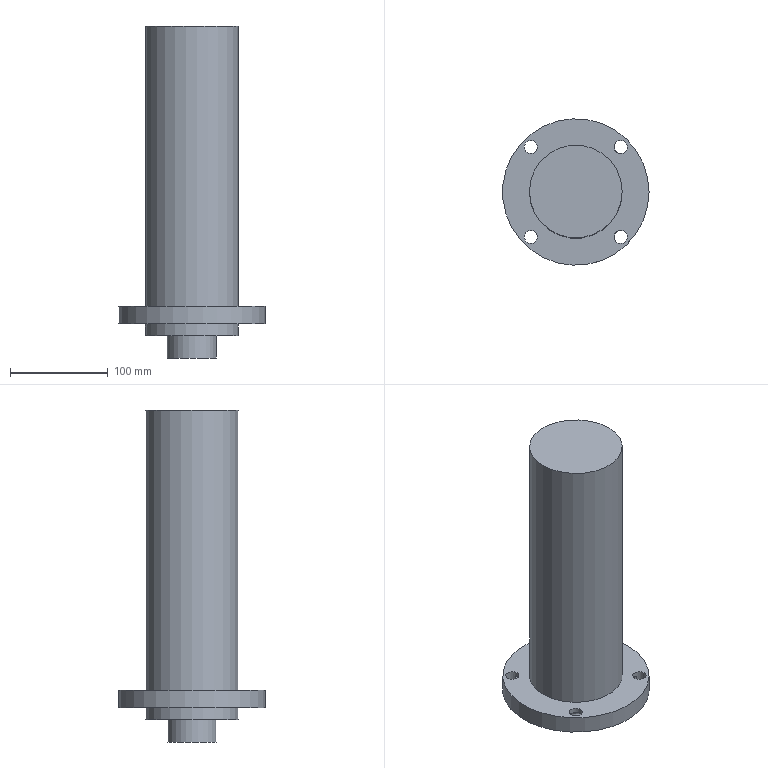Part | NX | features solid 2 | 1 solid | 14 faces | box 150 x 150 x 340 mm | volume 2465510 mm3 | cylinder 8 | plane 5 | torus 1 | commonest cylinder face diameters 13.5 x4 95 x2 50 x1 150 x1
STEP:
#1=CARTESIAN_POINT('',(955.75,441.,55.));
#2=VERTEX_POINT('',#1);
#3=CARTESIAN_POINT('',(949.,441.,55.));
#4=DIRECTION('',(0.,0.,1.));
#5=DIRECTION('',(1.,0.,0.));
#6=AXIS2_PLACEMENT_3D('',#3,#4,#5);
#7=CIRCLE('',#6,6.75);
#8=EDGE_CURVE('',#2,#2,#7,.F.);
#9=ORIENTED_EDGE('',*,*,#8,.T.);
#10=EDGE_LOOP('',(#9));
#11=FACE_BOUND('',#10,.T.);
#12=CARTESIAN_POINT('',(1047.75,349.,55.));
#13=VERTEX_POINT('',#12);
#14=CARTESIAN_POINT('',(1041.,349.,55.));
#15=DIRECTION('',(0.,0.,1.));
#16=DIRECTION('',(1.,0.,0.));
#17=AXIS2_PLACEMENT_3D('',#14,#15,#16);
#18=CIRCLE('',#17,6.75);
#19=EDGE_CURVE('',#13,#13,#18,.F.);
#20=ORIENTED_EDGE('',*,*,#19,.T.);
#21=EDGE_LOOP('',(#20));
#22=FACE_BOUND('',#21,.T.);
#23=CARTESIAN_POINT('',(1070.,395.,55.));
#24=VERTEX_POINT('',#23);
#25=CARTESIAN_POINT('',(995.,395.,55.));
#26=DIRECTION('',(0.,0.,1.));
#27=DIRECTION('',(1.,0.,0.));
#28=AXIS2_PLACEMENT_3D('',#25,#26,#27);
#29=CIRCLE('',#28,75.);
#30=EDGE_CURVE('',#24,#24,#29,.T.);
#31=ORIENTED_EDGE('',*,*,#30,.T.);
#32=EDGE_LOOP('',(#31));
#33=FACE_BOUND('',#32,.T.);
#34=CARTESIAN_POINT('',(1042.5,395.,55.));
#35=VERTEX_POINT('',#34);
#36=CARTESIAN_POINT('',(995.,395.,55.));
#37=DIRECTION('',(0.,0.,1.));
#38=DIRECTION('',(1.,0.,0.));
#39=AXIS2_PLACEMENT_3D('',#36,#37,#38);
#40=CIRCLE('',#39,47.5);
#41=EDGE_CURVE('',#35,#35,#40,.T.);
#42=ORIENTED_EDGE('',*,*,#41,.F.);
#43=EDGE_LOOP('',(#42));
#44=FACE_BOUND('',#43,.T.);
#45=CARTESIAN_POINT('',(1047.75,441.,55.));
#46=VERTEX_POINT('',#45);
#47=CARTESIAN_POINT('',(1041.,441.,55.));
#48=DIRECTION('',(0.,0.,1.));
#49=DIRECTION('',(1.,0.,0.));
#50=AXIS2_PLACEMENT_3D('',#47,#48,#49);
#51=CIRCLE('',#50,6.75);
#52=EDGE_CURVE('',#46,#46,#51,.F.);
#53=ORIENTED_EDGE('',*,*,#52,.T.);
#54=EDGE_LOOP('',(#53));
#55=FACE_BOUND('',#54,.T.);
#56=CARTESIAN_POINT('',(955.75,349.,55.));
#57=VERTEX_POINT('',#56);
#58=CARTESIAN_POINT('',(949.,349.,55.));
#59=DIRECTION('',(0.,0.,1.));
#60=DIRECTION('',(1.,0.,0.));
#61=AXIS2_PLACEMENT_3D('',#58,#59,#60);
#62=CIRCLE('',#61,6.75);
#63=EDGE_CURVE('',#57,#57,#62,.F.);
#64=ORIENTED_EDGE('',*,*,#63,.T.);
#65=EDGE_LOOP('',(#64));
#66=FACE_BOUND('',#65,.T.);
#67=CARTESIAN_POINT('',(995.,395.,55.));
#68=DIRECTION('',(0.,0.,-1.));
#69=DIRECTION('',(1.,0.,0.));
#70=AXIS2_PLACEMENT_3D('',#67,#68,#69);
#71=PLANE('',#70);
#72=ADVANCED_FACE('',(#11,#22,#33,#44,#55,#66),#71,.F.);
#73=CARTESIAN_POINT('',(955.75,441.,37.));
#74=VERTEX_POINT('',#73);
#75=CARTESIAN_POINT('',(949.,441.,37.));
#76=DIRECTION('',(0.,0.,1.));
#77=DIRECTION('',(1.,0.,0.));
#78=AXIS2_PLACEMENT_3D('',#75,#76,#77);
#79=CIRCLE('',#78,6.75);
#80=EDGE_CURVE('',#74,#74,#79,.F.);
#81=ORIENTED_EDGE('',*,*,#80,.F.);
#82=EDGE_LOOP('',(#81));
#83=FACE_BOUND('',#82,.T.);
#84=CARTESIAN_POINT('',(1047.75,349.,37.));
#85=VERTEX_POINT('',#84);
#86=CARTESIAN_POINT('',(1041.,349.,37.));
#87=DIRECTION('',(0.,0.,1.));
#88=DIRECTION('',(1.,0.,0.));
#89=AXIS2_PLACEMENT_3D('',#86,#87,#88);
#90=CIRCLE('',#89,6.75);
#91=EDGE_CURVE('',#85,#85,#90,.F.);
#92=ORIENTED_EDGE('',*,*,#91,.F.);
#93=EDGE_LOOP('',(#92));
#94=FACE_BOUND('',#93,.T.);
#95=CARTESIAN_POINT('',(1070.,395.,37.));
#96=VERTEX_POINT('',#95);
#97=CARTESIAN_POINT('',(995.,395.,37.));
#98=DIRECTION('',(0.,0.,1.));
#99=DIRECTION('',(1.,0.,0.));
#100=AXIS2_PLACEMENT_3D('',#97,#98,#99);
#101=CIRCLE('',#100,75.);
#102=EDGE_CURVE('',#96,#96,#101,.T.);
#103=ORIENTED_EDGE('',*,*,#102,.F.);
#104=EDGE_LOOP('',(#103));
#105=FACE_BOUND('',#104,.T.);
#106=CARTESIAN_POINT('',(1042.5,395.,37.));
#107=VERTEX_POINT('',#106);
#108=CARTESIAN_POINT('',(995.,395.,37.));
#109=DIRECTION('',(0.,0.,1.));
#110=DIRECTION('',(1.,0.,0.));
#111=AXIS2_PLACEMENT_3D('',#108,#109,#110);
#112=CIRCLE('',#111,47.5);
#113=EDGE_CURVE('',#107,#107,#112,.T.);
#114=ORIENTED_EDGE('',*,*,#113,.T.);
#115=EDGE_LOOP('',(#114));
#116=FACE_BOUND('',#115,.T.);
#117=CARTESIAN_POINT('',(1047.75,441.,37.));
#118=VERTEX_POINT('',#117);
#119=CARTESIAN_POINT('',(1041.,441.,37.));
#120=DIRECTION('',(0.,0.,1.));
#121=DIRECTION('',(1.,0.,0.));
#122=AXIS2_PLACEMENT_3D('',#119,#120,#121);
#123=CIRCLE('',#122,6.75);
#124=EDGE_CURVE('',#118,#118,#123,.F.);
#125=ORIENTED_EDGE('',*,*,#124,.F.);
#126=EDGE_LOOP('',(#125));
#127=FACE_BOUND('',#126,.T.);
#128=CARTESIAN_POINT('',(955.75,349.,37.));
#129=VERTEX_POINT('',#128);
#130=CARTESIAN_POINT('',(949.,349.,37.));
#131=DIRECTION('',(0.,0.,1.));
#132=DIRECTION('',(1.,0.,0.));
#133=AXIS2_PLACEMENT_3D('',#130,#131,#132);
#134=CIRCLE('',#133,6.75);
#135=EDGE_CURVE('',#129,#129,#134,.F.);
#136=ORIENTED_EDGE('',*,*,#135,.F.);
#137=EDGE_LOOP('',(#136));
#138=FACE_BOUND('',#137,.T.);
#139=CARTESIAN_POINT('',(995.,395.,37.));
#140=DIRECTION('',(0.,0.,-1.));
#141=DIRECTION('',(1.,0.,0.));
#142=AXIS2_PLACEMENT_3D('',#139,#140,#141);
#143=PLANE('',#142);
#144=ADVANCED_FACE('',(#83,#94,#105,#116,#127,#138),#143,.T.);
#145=CARTESIAN_POINT('',(946.897,434.586,48.486));
#146=VERTEX_POINT('',#145);
#147=CARTESIAN_POINT('',(946.677,434.627,46.069));
#148=CARTESIAN_POINT('',(946.547,434.691,48.675));
#149=CARTESIAN_POINT('',(948.515,434.126,50.145));
#150=CARTESIAN_POINT('',(950.871,434.386,49.961));
#151=CARTESIAN_POINT('',(952.868,435.318,49.355));
#152=CARTESIAN_POINT('',(954.541,436.93,49.301));
#153=CARTESIAN_POINT('',(955.542,438.899,49.902));
#154=CARTESIAN_POINT('',(955.893,441.218,50.179));
#155=CARTESIAN_POINT('',(955.373,443.323,48.93));
#156=CARTESIAN_POINT('',(955.309,443.454,46.328));
#157=CARTESIAN_POINT('',(955.874,441.486,44.855));
#158=CARTESIAN_POINT('',(955.615,439.129,45.039));
#159=CARTESIAN_POINT('',(954.683,437.133,45.644));
#160=CARTESIAN_POINT('',(953.072,435.46,45.699));
#161=CARTESIAN_POINT('',(951.103,434.459,45.098));
#162=CARTESIAN_POINT('',(948.782,434.107,44.821));
#163=CARTESIAN_POINT('',(946.677,434.627,46.069));
#164=CARTESIAN_POINT('',(946.547,434.691,48.675));
#165=CARTESIAN_POINT('',(948.515,434.126,50.145));
#166=B_SPLINE_CURVE_WITH_KNOTS('',3,(#147,#148,#149,#150,#151,#152,#153,#154,#155,#156,#157,#158,#159,#160,#161,#162,#163,#164,#165),.UNSPECIFIED.,.T.,.F.,(1,1,1,1,1,1,1,1,1,1,1,1,1,1,1,1,1,1,1,1,1,1,1),(-0.006805,-0.004537,-0.002268,0.,0.002268,0.004537,0.006805,0.009074,0.01134,0.01361,0.01588,0.01815,0.02042,0.02268,0.02495,0.02722,0.02949,0.03176,0.03403,0.03629,0.03856,0.04083,0.0431),.UNSPECIFIED.);
#167=EDGE_CURVE('',#146,#146,#166,.T.);
#168=ORIENTED_EDGE('',*,*,#167,.T.);
#169=EDGE_LOOP('',(#168));
#170=FACE_BOUND('',#169,.T.);
#171=CARTESIAN_POINT('',(1034.586,346.897,48.486));
#172=VERTEX_POINT('',#171);
#173=CARTESIAN_POINT('',(1034.125,348.515,50.146));
#174=CARTESIAN_POINT('',(1034.691,346.548,48.673));
#175=CARTESIAN_POINT('',(1034.628,346.675,46.075));
#176=CARTESIAN_POINT('',(1034.107,348.78,44.821));
#177=CARTESIAN_POINT('',(1034.457,351.097,45.097));
#178=CARTESIAN_POINT('',(1035.455,353.065,45.697));
#179=CARTESIAN_POINT('',(1037.125,354.677,45.647));
#180=CARTESIAN_POINT('',(1039.113,355.61,45.043));
#181=CARTESIAN_POINT('',(1041.473,355.876,44.855));
#182=CARTESIAN_POINT('',(1043.44,355.314,46.303));
#183=CARTESIAN_POINT('',(1043.337,355.367,48.91));
#184=CARTESIAN_POINT('',(1041.233,355.893,50.179));
#185=CARTESIAN_POINT('',(1038.91,355.546,49.905));
#186=CARTESIAN_POINT('',(1036.938,354.548,49.303));
#187=CARTESIAN_POINT('',(1035.323,352.877,49.353));
#188=CARTESIAN_POINT('',(1034.386,350.875,49.96));
#189=CARTESIAN_POINT('',(1034.125,348.515,50.146));
#190=CARTESIAN_POINT('',(1034.691,346.548,48.673));
#191=CARTESIAN_POINT('',(1034.628,346.675,46.075));
#192=B_SPLINE_CURVE_WITH_KNOTS('',3,(#173,#174,#175,#176,#177,#178,#179,#180,#181,#182,#183,#184,#185,#186,#187,#188,#189,#190,#191),.UNSPECIFIED.,.T.,.F.,(1,1,1,1,1,1,1,1,1,1,1,1,1,1,1,1,1,1,1,1,1,1,1),(-0.0068,-0.004534,-0.002267,0.,0.002267,0.004534,0.0068,0.009067,0.01133,0.0136,0.01587,0.01813,0.0204,0.02267,0.02493,0.0272,0.02947,0.03173,0.034,0.03627,0.03854,0.0408,0.04307),.UNSPECIFIED.);
#193=EDGE_CURVE('',#172,#172,#192,.T.);
#194=ORIENTED_EDGE('',*,*,#193,.T.);
#195=EDGE_LOOP('',(#194));
#196=FACE_BOUND('',#195,.T.);
#197=CARTESIAN_POINT('',(1035.627,436.915,49.398));
#198=VERTEX_POINT('',#197);
#199=CARTESIAN_POINT('',(1034.484,438.824,49.881));
#200=CARTESIAN_POINT('',(1035.516,436.85,49.282));
#201=CARTESIAN_POINT('',(1037.213,435.265,49.379));
#202=CARTESIAN_POINT('',(1039.218,434.359,49.982));
#203=CARTESIAN_POINT('',(1041.588,434.136,50.124));
#204=CARTESIAN_POINT('',(1043.489,434.711,48.581));
#205=CARTESIAN_POINT('',(1043.274,434.603,45.985));
#206=CARTESIAN_POINT('',(1041.117,434.104,44.813));
#207=CARTESIAN_POINT('',(1038.824,434.485,45.119));
#208=CARTESIAN_POINT('',(1036.864,435.506,45.715));
#209=CARTESIAN_POINT('',(1035.269,437.204,45.624));
#210=CARTESIAN_POINT('',(1034.362,439.21,45.019));
#211=CARTESIAN_POINT('',(1034.135,441.58,44.873));
#212=CARTESIAN_POINT('',(1034.71,443.489,46.416));
#213=CARTESIAN_POINT('',(1034.604,443.275,49.014));
#214=CARTESIAN_POINT('',(1034.104,441.116,50.187));
#215=CARTESIAN_POINT('',(1034.484,438.824,49.881));
#216=CARTESIAN_POINT('',(1035.516,436.85,49.282));
#217=CARTESIAN_POINT('',(1037.213,435.265,49.379));
#218=B_SPLINE_CURVE_WITH_KNOTS('',3,(#199,#200,#201,#202,#203,#204,#205,#206,#207,#208,#209,#210,#211,#212,#213,#214,#215,#216,#217),.UNSPECIFIED.,.T.,.F.,(1,1,1,1,1,1,1,1,1,1,1,1,1,1,1,1,1,1,1,1,1,1,1),(-0.006763,-0.004509,-0.002254,0.,0.002254,0.004509,0.006763,0.009018,0.01127,0.01353,0.01578,0.01804,0.02029,0.02254,0.0248,0.02705,0.02931,0.03156,0.03382,0.03607,0.03833,0.04058,0.04284),.UNSPECIFIED.);
#219=EDGE_CURVE('',#198,#198,#218,.T.);
#220=ORIENTED_EDGE('',*,*,#219,.T.);
#221=EDGE_LOOP('',(#220));
#222=FACE_BOUND('',#221,.T.);
#223=CARTESIAN_POINT('',(946.897,355.414,48.486));
#224=VERTEX_POINT('',#223);
#225=CARTESIAN_POINT('',(948.515,355.875,50.146));
#226=CARTESIAN_POINT('',(946.548,355.309,48.673));
#227=CARTESIAN_POINT('',(946.675,355.372,46.075));
#228=CARTESIAN_POINT('',(948.78,355.893,44.821));
#229=CARTESIAN_POINT('',(951.097,355.543,45.097));
#230=CARTESIAN_POINT('',(953.065,354.545,45.697));
#231=CARTESIAN_POINT('',(954.677,352.875,45.647));
#232=CARTESIAN_POINT('',(955.61,350.887,45.043));
#233=CARTESIAN_POINT('',(955.876,348.527,44.855));
#234=CARTESIAN_POINT('',(955.314,346.56,46.303));
#235=CARTESIAN_POINT('',(955.367,346.663,48.91));
#236=CARTESIAN_POINT('',(955.893,348.767,50.179));
#237=CARTESIAN_POINT('',(955.546,351.09,49.905));
#238=CARTESIAN_POINT('',(954.548,353.062,49.303));
#239=CARTESIAN_POINT('',(952.877,354.677,49.353));
#240=CARTESIAN_POINT('',(950.875,355.614,49.96));
#241=CARTESIAN_POINT('',(948.515,355.875,50.146));
#242=CARTESIAN_POINT('',(946.548,355.309,48.673));
#243=CARTESIAN_POINT('',(946.675,355.372,46.075));
#244=B_SPLINE_CURVE_WITH_KNOTS('',3,(#225,#226,#227,#228,#229,#230,#231,#232,#233,#234,#235,#236,#237,#238,#239,#240,#241,#242,#243),.UNSPECIFIED.,.T.,.F.,(1,1,1,1,1,1,1,1,1,1,1,1,1,1,1,1,1,1,1,1,1,1,1),(-0.0068,-0.004534,-0.002267,0.,0.002267,0.004534,0.0068,0.009067,0.01133,0.0136,0.01587,0.01813,0.0204,0.02267,0.02493,0.0272,0.02947,0.03173,0.034,0.03627,0.03854,0.0408,0.04307),.UNSPECIFIED.);
#245=EDGE_CURVE('',#224,#224,#244,.T.);
#246=ORIENTED_EDGE('',*,*,#245,.T.);
#247=EDGE_LOOP('',(#246));
#248=FACE_BOUND('',#247,.T.);
#249=CARTESIAN_POINT('',(995.,395.,47.5));
#250=DIRECTION('',(0.,0.,-1.));
#251=DIRECTION('',(1.,0.,0.));
#252=AXIS2_PLACEMENT_3D('',#249,#250,#251);
#253=TOROIDAL_SURFACE('',#252,60.,2.5);
#254=ADVANCED_FACE('',(#170,#196,#222,#248),#253,.F.);
#255=CARTESIAN_POINT('',(947.5,395.,342.));
#256=VERTEX_POINT('',#255);
#257=CARTESIAN_POINT('',(995.,395.,342.));
#258=DIRECTION('',(0.,0.,-1.));
#259=DIRECTION('',(-1.,0.,0.));
#260=AXIS2_PLACEMENT_3D('',#257,#258,#259);
#261=CIRCLE('',#260,47.5);
#262=EDGE_CURVE('',#256,#256,#261,.F.);
#263=ORIENTED_EDGE('',*,*,#262,.F.);
#264=EDGE_LOOP('',(#263));
#265=FACE_BOUND('',#264,.T.);
#266=ORIENTED_EDGE('',*,*,#41,.T.);
#267=EDGE_LOOP('',(#266));
#268=FACE_BOUND('',#267,.T.);
#269=CARTESIAN_POINT('',(995.,395.,127.));
#270=DIRECTION('',(0.,0.,-1.));
#271=DIRECTION('',(1.,0.,0.));
#272=AXIS2_PLACEMENT_3D('',#269,#270,#271);
#273=CYLINDRICAL_SURFACE('',#272,47.5);
#274=ADVANCED_FACE('',(#265,#268),#273,.T.);
#275=ORIENTED_EDGE('',*,*,#262,.T.);
#276=EDGE_LOOP('',(#275));
#277=FACE_BOUND('',#276,.T.);
#278=CARTESIAN_POINT('',(995.,455.,342.));
#279=DIRECTION('',(0.,0.,-1.));
#280=DIRECTION('',(1.,0.,0.));
#281=AXIS2_PLACEMENT_3D('',#278,#279,#280);
#282=PLANE('',#281);
#283=ADVANCED_FACE('',(#277),#282,.F.);
#284=ORIENTED_EDGE('',*,*,#102,.T.);
#285=EDGE_LOOP('',(#284));
#286=FACE_BOUND('',#285,.T.);
#287=ORIENTED_EDGE('',*,*,#30,.F.);
#288=EDGE_LOOP('',(#287));
#289=FACE_BOUND('',#288,.T.);
#290=CARTESIAN_POINT('',(995.,395.,47.5));
#291=DIRECTION('',(0.,0.,-1.));
#292=DIRECTION('',(1.,0.,0.));
#293=AXIS2_PLACEMENT_3D('',#290,#291,#292);
#294=CYLINDRICAL_SURFACE('',#293,75.);
#295=ADVANCED_FACE('',(#286,#289),#294,.T.);
#296=CARTESIAN_POINT('',(970.,395.,2.));
#297=VERTEX_POINT('',#296);
#298=CARTESIAN_POINT('',(995.,395.,2.));
#299=DIRECTION('',(0.,0.,-1.));
#300=DIRECTION('',(-1.,0.,0.));
#301=AXIS2_PLACEMENT_3D('',#298,#299,#300);
#302=CIRCLE('',#301,25.);
#303=EDGE_CURVE('',#297,#297,#302,.F.);
#304=ORIENTED_EDGE('',*,*,#303,.F.);
#305=EDGE_LOOP('',(#304));
#306=FACE_BOUND('',#305,.T.);
#307=CARTESIAN_POINT('',(995.,395.,2.));
#308=DIRECTION('',(0.,0.,-1.));
#309=DIRECTION('',(1.,0.,0.));
#310=AXIS2_PLACEMENT_3D('',#307,#308,#309);
#311=PLANE('',#310);
#312=ADVANCED_FACE('',(#306),#311,.T.);
#313=CARTESIAN_POINT('',(1020.,395.,25.));
#314=VERTEX_POINT('',#313);
#315=CARTESIAN_POINT('',(995.,395.,25.));
#316=DIRECTION('',(0.,0.,1.));
#317=DIRECTION('',(1.,0.,0.));
#318=AXIS2_PLACEMENT_3D('',#315,#316,#317);
#319=CIRCLE('',#318,25.);
#320=EDGE_CURVE('',#314,#314,#319,.T.);
#321=ORIENTED_EDGE('',*,*,#320,.F.);
#322=EDGE_LOOP('',(#321));
#323=FACE_BOUND('',#322,.T.);
#324=ORIENTED_EDGE('',*,*,#303,.T.);
#325=EDGE_LOOP('',(#324));
#326=FACE_BOUND('',#325,.T.);
#327=CARTESIAN_POINT('',(995.,395.,127.));
#328=DIRECTION('',(0.,0.,-1.));
#329=DIRECTION('',(1.,0.,0.));
#330=AXIS2_PLACEMENT_3D('',#327,#328,#329);
#331=CYLINDRICAL_SURFACE('',#330,25.);
#332=ADVANCED_FACE('',(#323,#326),#331,.T.);
#333=CARTESIAN_POINT('',(1042.5,395.,25.));
#334=VERTEX_POINT('',#333);
#335=CARTESIAN_POINT('',(995.,395.,25.));
#336=DIRECTION('',(0.,0.,1.));
#337=DIRECTION('',(1.,0.,0.));
#338=AXIS2_PLACEMENT_3D('',#335,#336,#337);
#339=CIRCLE('',#338,47.5);
#340=EDGE_CURVE('',#334,#334,#339,.T.);
#341=ORIENTED_EDGE('',*,*,#340,.F.);
#342=EDGE_LOOP('',(#341));
#343=FACE_BOUND('',#342,.T.);
#344=ORIENTED_EDGE('',*,*,#320,.T.);
#345=EDGE_LOOP('',(#344));
#346=FACE_BOUND('',#345,.T.);
#347=CARTESIAN_POINT('',(995.,427.5,25.));
#348=DIRECTION('',(0.,0.,-1.));
#349=DIRECTION('',(1.,0.,0.));
#350=AXIS2_PLACEMENT_3D('',#347,#348,#349);
#351=PLANE('',#350);
#352=ADVANCED_FACE('',(#343,#346),#351,.T.);
#353=ORIENTED_EDGE('',*,*,#113,.F.);
#354=EDGE_LOOP('',(#353));
#355=FACE_BOUND('',#354,.T.);
#356=ORIENTED_EDGE('',*,*,#340,.T.);
#357=EDGE_LOOP('',(#356));
#358=FACE_BOUND('',#357,.T.);
#359=CARTESIAN_POINT('',(995.,395.,127.));
#360=DIRECTION('',(0.,0.,-1.));
#361=DIRECTION('',(1.,0.,0.));
#362=AXIS2_PLACEMENT_3D('',#359,#360,#361);
#363=CYLINDRICAL_SURFACE('',#362,47.5);
#364=ADVANCED_FACE('',(#355,#358),#363,.T.);
#365=ORIENTED_EDGE('',*,*,#193,.F.);
#366=EDGE_LOOP('',(#365));
#367=FACE_BOUND('',#366,.T.);
#368=ORIENTED_EDGE('',*,*,#91,.T.);
#369=EDGE_LOOP('',(#368));
#370=FACE_BOUND('',#369,.T.);
#371=ORIENTED_EDGE('',*,*,#19,.F.);
#372=EDGE_LOOP('',(#371));
#373=FACE_BOUND('',#372,.T.);
#374=CARTESIAN_POINT('',(1041.,349.,36.));
#375=DIRECTION('',(0.,0.,1.));
#376=DIRECTION('',(-1.,0.,0.));
#377=AXIS2_PLACEMENT_3D('',#374,#375,#376);
#378=CYLINDRICAL_SURFACE('',#377,6.75);
#379=ADVANCED_FACE('',(#367,#370,#373),#378,.F.);
#380=ORIENTED_EDGE('',*,*,#219,.F.);
#381=EDGE_LOOP('',(#380));
#382=FACE_BOUND('',#381,.T.);
#383=ORIENTED_EDGE('',*,*,#124,.T.);
#384=EDGE_LOOP('',(#383));
#385=FACE_BOUND('',#384,.T.);
#386=ORIENTED_EDGE('',*,*,#52,.F.);
#387=EDGE_LOOP('',(#386));
#388=FACE_BOUND('',#387,.T.);
#389=CARTESIAN_POINT('',(1041.,441.,36.));
#390=DIRECTION('',(0.,0.,1.));
#391=DIRECTION('',(-1.,0.,0.));
#392=AXIS2_PLACEMENT_3D('',#389,#390,#391);
#393=CYLINDRICAL_SURFACE('',#392,6.75);
#394=ADVANCED_FACE('',(#382,#385,#388),#393,.F.);
#395=ORIENTED_EDGE('',*,*,#167,.F.);
#396=EDGE_LOOP('',(#395));
#397=FACE_BOUND('',#396,.T.);
#398=ORIENTED_EDGE('',*,*,#80,.T.);
#399=EDGE_LOOP('',(#398));
#400=FACE_BOUND('',#399,.T.);
#401=ORIENTED_EDGE('',*,*,#8,.F.);
#402=EDGE_LOOP('',(#401));
#403=FACE_BOUND('',#402,.T.);
#404=CARTESIAN_POINT('',(949.,441.,36.));
#405=DIRECTION('',(0.,0.,1.));
#406=DIRECTION('',(-1.,0.,0.));
#407=AXIS2_PLACEMENT_3D('',#404,#405,#406);
#408=CYLINDRICAL_SURFACE('',#407,6.75);
#409=ADVANCED_FACE('',(#397,#400,#403),#408,.F.);
#410=ORIENTED_EDGE('',*,*,#245,.F.);
#411=EDGE_LOOP('',(#410));
#412=FACE_BOUND('',#411,.T.);
#413=ORIENTED_EDGE('',*,*,#135,.T.);
#414=EDGE_LOOP('',(#413));
#415=FACE_BOUND('',#414,.T.);
#416=ORIENTED_EDGE('',*,*,#63,.F.);
#417=EDGE_LOOP('',(#416));
#418=FACE_BOUND('',#417,.T.);
#419=CARTESIAN_POINT('',(949.,349.,36.));
#420=DIRECTION('',(0.,0.,1.));
#421=DIRECTION('',(-1.,0.,0.));
#422=AXIS2_PLACEMENT_3D('',#419,#420,#421);
#423=CYLINDRICAL_SURFACE('',#422,6.75);
#424=ADVANCED_FACE('',(#412,#415,#418),#423,.F.);
#425=CLOSED_SHELL('',(#72,#144,#254,#274,#283,#295,#312,#332,#352,#364,#379,#394,#409,#424));
#426=MANIFOLD_SOLID_BREP('',#425);
#427=(LENGTH_UNIT()NAMED_UNIT(*)SI_UNIT(.MILLI.,.METRE.));
#428=UNCERTAINTY_MEASURE_WITH_UNIT(LENGTH_MEASURE(0.0508),#427,'','');
#429=(NAMED_UNIT(*)PLANE_ANGLE_UNIT()SI_UNIT($,.RADIAN.));
#430=(NAMED_UNIT(*)SI_UNIT($,.STERADIAN.)SOLID_ANGLE_UNIT());
#431=(GEOMETRIC_REPRESENTATION_CONTEXT(3)GLOBAL_UNCERTAINTY_ASSIGNED_CONTEXT((#428))GLOBAL_UNIT_ASSIGNED_CONTEXT((#427,#429,#430))REPRESENTATION_CONTEXT('',''));
#432=ADVANCED_BREP_SHAPE_REPRESENTATION('',(#426),#431);